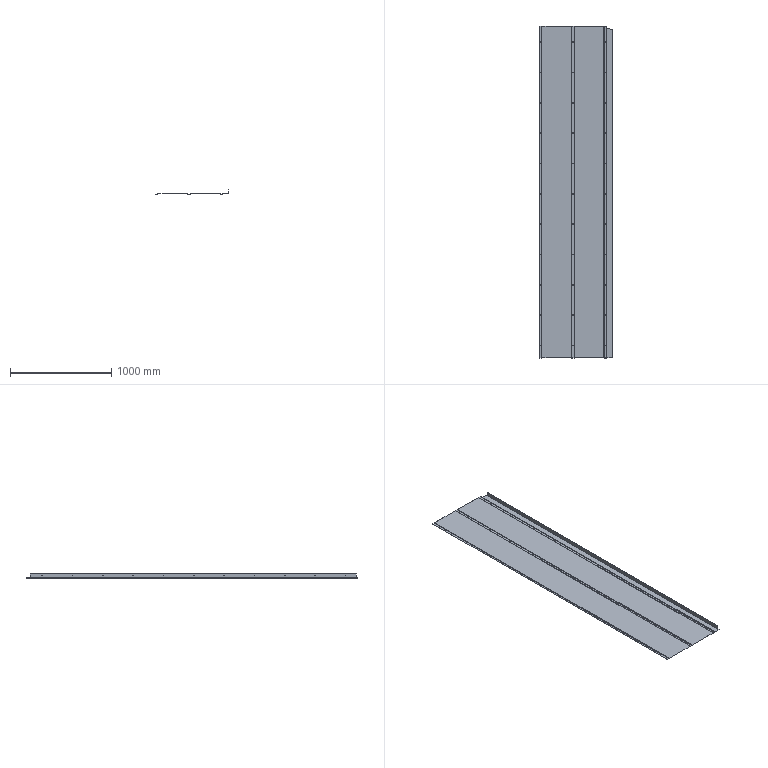Part | STEP file | TS-S83 | 1 solid | 191 faces | box 720 x 3283 x 43 mm | volume 3005343 mm3 | cylinder 113 | plane 78 | commonest cylinder face diameters 5.4 x88 0.4 x11 2.8 x11 10 x1 14 x1 16 x1